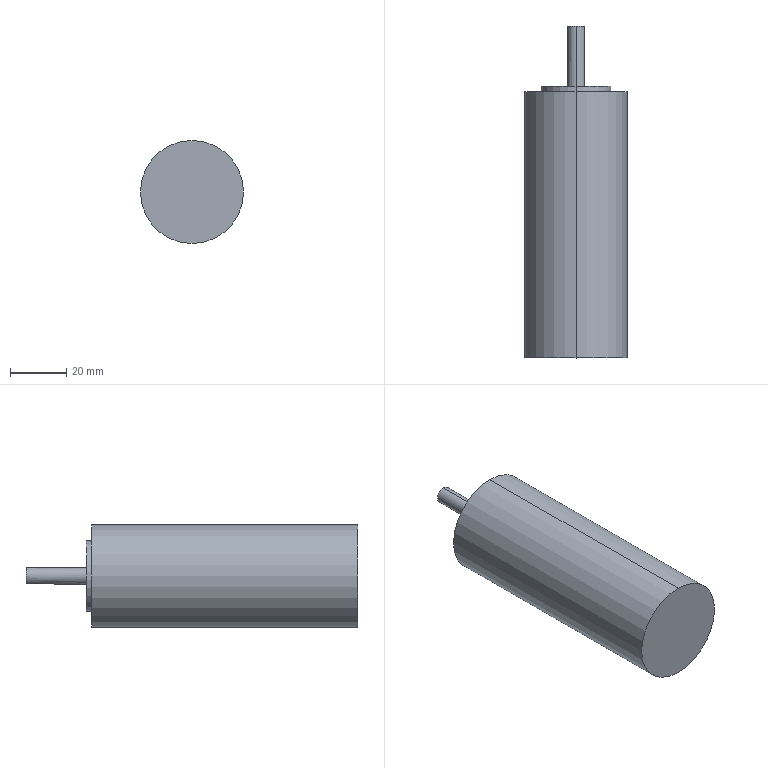Part | 1 solid | 12 faces | box 36.8 x 118.5 x 36.8 mm | volume 102622 mm3 | cylinder 6 | plane 6 | commonest cylinder face diameters 6 x2 25 x2 36.8 x2
STEP:
#1=CARTESIAN_POINT('',(0.,97.,12.5));
#2=VERTEX_POINT('',#1);
#3=CARTESIAN_POINT('',(0.,97.,-12.5));
#4=VERTEX_POINT('',#3);
#5=CARTESIAN_POINT('',(0.,97.,0.));
#6=DIRECTION('',(0.,1.,0.));
#7=DIRECTION('',(0.,0.,1.));
#8=AXIS2_PLACEMENT_3D('',#5,#6,#7);
#9=CIRCLE('',#8,12.5);
#10=EDGE_CURVE('',#2,#4,#9,.T.);
#11=ORIENTED_EDGE('',*,*,#10,.F.);
#12=CARTESIAN_POINT('',(0.,95.,12.5));
#13=VERTEX_POINT('',#12);
#14=CARTESIAN_POINT('',(0.,97.,12.5));
#15=DIRECTION('',(0.,-1.,0.));
#16=VECTOR('',#15,1000.);
#17=LINE('',#14,#16);
#18=EDGE_CURVE('',#2,#13,#17,.T.);
#19=ORIENTED_EDGE('',*,*,#18,.T.);
#20=CARTESIAN_POINT('',(0.,95.,-12.5));
#21=VERTEX_POINT('',#20);
#22=CARTESIAN_POINT('',(0.,95.,0.));
#23=DIRECTION('',(0.,1.,0.));
#24=DIRECTION('',(0.,0.,1.));
#25=AXIS2_PLACEMENT_3D('',#22,#23,#24);
#26=CIRCLE('',#25,12.5);
#27=EDGE_CURVE('',#13,#21,#26,.T.);
#28=ORIENTED_EDGE('',*,*,#27,.T.);
#29=CARTESIAN_POINT('',(0.,97.,-12.5));
#30=DIRECTION('',(0.,-1.,0.));
#31=VECTOR('',#30,1000.);
#32=LINE('',#29,#31);
#33=EDGE_CURVE('',#4,#21,#32,.T.);
#34=ORIENTED_EDGE('',*,*,#33,.F.);
#35=EDGE_LOOP('',(#11,#19,#28,#34));
#36=FACE_OUTER_BOUND('',#35,.T.);
#37=CARTESIAN_POINT('',(0.,97.,0.));
#38=DIRECTION('',(0.,-1.,0.));
#39=DIRECTION('',(0.,0.,-1.));
#40=AXIS2_PLACEMENT_3D('',#37,#38,#39);
#41=CYLINDRICAL_SURFACE('',#40,12.5);
#42=ADVANCED_FACE('',(#36),#41,.T.);
#43=CARTESIAN_POINT('',(0.,95.,18.4));
#44=VERTEX_POINT('',#43);
#45=CARTESIAN_POINT('',(0.,95.,-18.4));
#46=VERTEX_POINT('',#45);
#47=CARTESIAN_POINT('',(0.,95.,0.));
#48=DIRECTION('',(0.,1.,0.));
#49=DIRECTION('',(0.,0.,1.));
#50=AXIS2_PLACEMENT_3D('',#47,#48,#49);
#51=CIRCLE('',#50,18.4);
#52=EDGE_CURVE('',#44,#46,#51,.T.);
#53=ORIENTED_EDGE('',*,*,#52,.F.);
#54=CARTESIAN_POINT('',(0.,0.,18.4));
#55=VERTEX_POINT('',#54);
#56=CARTESIAN_POINT('',(0.,95.,18.4));
#57=DIRECTION('',(0.,-1.,0.));
#58=VECTOR('',#57,1000.);
#59=LINE('',#56,#58);
#60=EDGE_CURVE('',#44,#55,#59,.T.);
#61=ORIENTED_EDGE('',*,*,#60,.T.);
#62=CARTESIAN_POINT('',(0.,0.,-18.4));
#63=VERTEX_POINT('',#62);
#64=CARTESIAN_POINT('',(0.,0.,0.));
#65=DIRECTION('',(0.,1.,0.));
#66=DIRECTION('',(0.,0.,1.));
#67=AXIS2_PLACEMENT_3D('',#64,#65,#66);
#68=CIRCLE('',#67,18.4);
#69=EDGE_CURVE('',#55,#63,#68,.T.);
#70=ORIENTED_EDGE('',*,*,#69,.T.);
#71=CARTESIAN_POINT('',(0.,95.,-18.4));
#72=DIRECTION('',(0.,-1.,0.));
#73=VECTOR('',#72,1000.);
#74=LINE('',#71,#73);
#75=EDGE_CURVE('',#46,#63,#74,.T.);
#76=ORIENTED_EDGE('',*,*,#75,.F.);
#77=EDGE_LOOP('',(#53,#61,#70,#76));
#78=FACE_OUTER_BOUND('',#77,.T.);
#79=CARTESIAN_POINT('',(0.,95.,0.));
#80=DIRECTION('',(0.,-1.,0.));
#81=DIRECTION('',(0.,0.,-1.));
#82=AXIS2_PLACEMENT_3D('',#79,#80,#81);
#83=CYLINDRICAL_SURFACE('',#82,18.4);
#84=ADVANCED_FACE('',(#78),#83,.T.);
#85=CARTESIAN_POINT('',(0.,118.5,3.));
#86=VERTEX_POINT('',#85);
#87=CARTESIAN_POINT('',(1.658,118.5,-2.5));
#88=VERTEX_POINT('',#87);
#89=CARTESIAN_POINT('',(0.,118.5,0.));
#90=DIRECTION('',(0.,1.,0.));
#91=DIRECTION('',(0.,0.,1.));
#92=AXIS2_PLACEMENT_3D('',#89,#90,#91);
#93=CIRCLE('',#92,3.);
#94=EDGE_CURVE('',#86,#88,#93,.T.);
#95=ORIENTED_EDGE('',*,*,#94,.F.);
#96=CARTESIAN_POINT('',(0.,97.,3.));
#97=VERTEX_POINT('',#96);
#98=CARTESIAN_POINT('',(0.,118.5,3.));
#99=DIRECTION('',(0.,-1.,0.));
#100=VECTOR('',#99,1000.);
#101=LINE('',#98,#100);
#102=EDGE_CURVE('',#86,#97,#101,.T.);
#103=ORIENTED_EDGE('',*,*,#102,.T.);
#104=CARTESIAN_POINT('',(0.,97.,-3.));
#105=VERTEX_POINT('',#104);
#106=CARTESIAN_POINT('',(0.,97.,0.));
#107=DIRECTION('',(0.,1.,0.));
#108=DIRECTION('',(0.,0.,1.));
#109=AXIS2_PLACEMENT_3D('',#106,#107,#108);
#110=CIRCLE('',#109,3.);
#111=EDGE_CURVE('',#97,#105,#110,.T.);
#112=ORIENTED_EDGE('',*,*,#111,.T.);
#113=CARTESIAN_POINT('',(0.,108.5,-3.));
#114=VERTEX_POINT('',#113);
#115=CARTESIAN_POINT('',(0.,118.5,-3.));
#116=DIRECTION('',(0.,-1.,0.));
#117=VECTOR('',#116,1000.);
#118=LINE('',#115,#117);
#119=EDGE_CURVE('',#114,#105,#118,.T.);
#120=ORIENTED_EDGE('',*,*,#119,.F.);
#121=CARTESIAN_POINT('',(1.658,108.5,-2.5));
#122=VERTEX_POINT('',#121);
#123=CARTESIAN_POINT('',(0.,108.5,0.));
#124=DIRECTION('',(0.,1.,0.));
#125=DIRECTION('',(0.,0.,1.));
#126=AXIS2_PLACEMENT_3D('',#123,#124,#125);
#127=CIRCLE('',#126,3.);
#128=EDGE_CURVE('',#122,#114,#127,.T.);
#129=ORIENTED_EDGE('',*,*,#128,.F.);
#130=CARTESIAN_POINT('',(1.658,108.5,-2.5));
#131=DIRECTION('',(0.,1.,0.));
#132=VECTOR('',#131,1000.);
#133=LINE('',#130,#132);
#134=EDGE_CURVE('',#122,#88,#133,.T.);
#135=ORIENTED_EDGE('',*,*,#134,.T.);
#136=EDGE_LOOP('',(#95,#103,#112,#120,#129,#135));
#137=FACE_OUTER_BOUND('',#136,.T.);
#138=CARTESIAN_POINT('',(0.,118.5,0.));
#139=DIRECTION('',(0.,-1.,0.));
#140=DIRECTION('',(0.,0.,-1.));
#141=AXIS2_PLACEMENT_3D('',#138,#139,#140);
#142=CYLINDRICAL_SURFACE('',#141,3.);
#143=ADVANCED_FACE('',(#137),#142,.T.);
#144=ORIENTED_EDGE('',*,*,#102,.F.);
#145=CARTESIAN_POINT('',(-1.658,118.5,-2.5));
#146=VERTEX_POINT('',#145);
#147=CARTESIAN_POINT('',(0.,118.5,0.));
#148=DIRECTION('',(0.,1.,0.));
#149=DIRECTION('',(0.,0.,1.));
#150=AXIS2_PLACEMENT_3D('',#147,#148,#149);
#151=CIRCLE('',#150,3.);
#152=EDGE_CURVE('',#146,#86,#151,.T.);
#153=ORIENTED_EDGE('',*,*,#152,.F.);
#154=CARTESIAN_POINT('',(-1.658,108.5,-2.5));
#155=VERTEX_POINT('',#154);
#156=CARTESIAN_POINT('',(-1.658,108.5,-2.5));
#157=DIRECTION('',(0.,1.,0.));
#158=VECTOR('',#157,1000.);
#159=LINE('',#156,#158);
#160=EDGE_CURVE('',#155,#146,#159,.T.);
#161=ORIENTED_EDGE('',*,*,#160,.F.);
#162=CARTESIAN_POINT('',(0.,108.5,0.));
#163=DIRECTION('',(0.,1.,0.));
#164=DIRECTION('',(0.,0.,1.));
#165=AXIS2_PLACEMENT_3D('',#162,#163,#164);
#166=CIRCLE('',#165,3.);
#167=EDGE_CURVE('',#114,#155,#166,.T.);
#168=ORIENTED_EDGE('',*,*,#167,.F.);
#169=ORIENTED_EDGE('',*,*,#119,.T.);
#170=CARTESIAN_POINT('',(0.,97.,0.));
#171=DIRECTION('',(0.,1.,0.));
#172=DIRECTION('',(0.,0.,1.));
#173=AXIS2_PLACEMENT_3D('',#170,#171,#172);
#174=CIRCLE('',#173,3.);
#175=EDGE_CURVE('',#105,#97,#174,.T.);
#176=ORIENTED_EDGE('',*,*,#175,.T.);
#177=EDGE_LOOP('',(#144,#153,#161,#168,#169,#176));
#178=FACE_OUTER_BOUND('',#177,.T.);
#179=CARTESIAN_POINT('',(0.,118.5,0.));
#180=DIRECTION('',(0.,-1.,0.));
#181=DIRECTION('',(0.,0.,-1.));
#182=AXIS2_PLACEMENT_3D('',#179,#180,#181);
#183=CYLINDRICAL_SURFACE('',#182,3.);
#184=ADVANCED_FACE('',(#178),#183,.T.);
#185=ORIENTED_EDGE('',*,*,#152,.T.);
#186=ORIENTED_EDGE('',*,*,#94,.T.);
#187=CARTESIAN_POINT('',(-1.658,118.5,-2.5));
#188=DIRECTION('',(-1.,0.,0.));
#189=VECTOR('',#188,1000.);
#190=LINE('',#187,#189);
#191=EDGE_CURVE('',#88,#146,#190,.T.);
#192=ORIENTED_EDGE('',*,*,#191,.T.);
#193=EDGE_LOOP('',(#185,#186,#192));
#194=FACE_OUTER_BOUND('',#193,.T.);
#195=CARTESIAN_POINT('',(0.,118.5,0.));
#196=DIRECTION('',(0.,1.,0.));
#197=DIRECTION('',(0.,0.,1.));
#198=AXIS2_PLACEMENT_3D('',#195,#196,#197);
#199=PLANE('',#198);
#200=ADVANCED_FACE('',(#194),#199,.T.);
#201=ORIENTED_EDGE('',*,*,#60,.F.);
#202=CARTESIAN_POINT('',(0.,95.,0.));
#203=DIRECTION('',(0.,1.,0.));
#204=DIRECTION('',(0.,0.,1.));
#205=AXIS2_PLACEMENT_3D('',#202,#203,#204);
#206=CIRCLE('',#205,18.4);
#207=EDGE_CURVE('',#46,#44,#206,.T.);
#208=ORIENTED_EDGE('',*,*,#207,.F.);
#209=ORIENTED_EDGE('',*,*,#75,.T.);
#210=CARTESIAN_POINT('',(0.,0.,0.));
#211=DIRECTION('',(0.,1.,0.));
#212=DIRECTION('',(0.,0.,1.));
#213=AXIS2_PLACEMENT_3D('',#210,#211,#212);
#214=CIRCLE('',#213,18.4);
#215=EDGE_CURVE('',#63,#55,#214,.T.);
#216=ORIENTED_EDGE('',*,*,#215,.T.);
#217=EDGE_LOOP('',(#201,#208,#209,#216));
#218=FACE_OUTER_BOUND('',#217,.T.);
#219=CARTESIAN_POINT('',(0.,95.,0.));
#220=DIRECTION('',(0.,-1.,0.));
#221=DIRECTION('',(0.,0.,-1.));
#222=AXIS2_PLACEMENT_3D('',#219,#220,#221);
#223=CYLINDRICAL_SURFACE('',#222,18.4);
#224=ADVANCED_FACE('',(#218),#223,.T.);
#225=CARTESIAN_POINT('',(0.,95.,0.));
#226=DIRECTION('',(0.,1.,0.));
#227=DIRECTION('',(0.,0.,1.));
#228=AXIS2_PLACEMENT_3D('',#225,#226,#227);
#229=CIRCLE('',#228,12.5);
#230=EDGE_CURVE('',#21,#13,#229,.T.);
#231=ORIENTED_EDGE('',*,*,#230,.F.);
#232=ORIENTED_EDGE('',*,*,#27,.F.);
#233=EDGE_LOOP('',(#231,#232));
#234=FACE_BOUND('',#233,.T.);
#235=ORIENTED_EDGE('',*,*,#207,.T.);
#236=ORIENTED_EDGE('',*,*,#52,.T.);
#237=EDGE_LOOP('',(#235,#236));
#238=FACE_OUTER_BOUND('',#237,.T.);
#239=CARTESIAN_POINT('',(0.,95.,0.));
#240=DIRECTION('',(0.,1.,0.));
#241=DIRECTION('',(0.,0.,1.));
#242=AXIS2_PLACEMENT_3D('',#239,#240,#241);
#243=PLANE('',#242);
#244=ADVANCED_FACE('',(#234,#238),#243,.T.);
#245=ORIENTED_EDGE('',*,*,#215,.F.);
#246=ORIENTED_EDGE('',*,*,#69,.F.);
#247=EDGE_LOOP('',(#245,#246));
#248=FACE_OUTER_BOUND('',#247,.T.);
#249=CARTESIAN_POINT('',(0.,0.,0.));
#250=DIRECTION('',(0.,1.,0.));
#251=DIRECTION('',(0.,0.,1.));
#252=AXIS2_PLACEMENT_3D('',#249,#250,#251);
#253=PLANE('',#252);
#254=ADVANCED_FACE('',(#248),#253,.F.);
#255=ORIENTED_EDGE('',*,*,#18,.F.);
#256=CARTESIAN_POINT('',(0.,97.,0.));
#257=DIRECTION('',(0.,1.,0.));
#258=DIRECTION('',(0.,0.,1.));
#259=AXIS2_PLACEMENT_3D('',#256,#257,#258);
#260=CIRCLE('',#259,12.5);
#261=EDGE_CURVE('',#4,#2,#260,.T.);
#262=ORIENTED_EDGE('',*,*,#261,.F.);
#263=ORIENTED_EDGE('',*,*,#33,.T.);
#264=ORIENTED_EDGE('',*,*,#230,.T.);
#265=EDGE_LOOP('',(#255,#262,#263,#264));
#266=FACE_OUTER_BOUND('',#265,.T.);
#267=CARTESIAN_POINT('',(0.,97.,0.));
#268=DIRECTION('',(0.,-1.,0.));
#269=DIRECTION('',(0.,0.,-1.));
#270=AXIS2_PLACEMENT_3D('',#267,#268,#269);
#271=CYLINDRICAL_SURFACE('',#270,12.5);
#272=ADVANCED_FACE('',(#266),#271,.T.);
#273=ORIENTED_EDGE('',*,*,#175,.F.);
#274=ORIENTED_EDGE('',*,*,#111,.F.);
#275=EDGE_LOOP('',(#273,#274));
#276=FACE_BOUND('',#275,.T.);
#277=ORIENTED_EDGE('',*,*,#261,.T.);
#278=ORIENTED_EDGE('',*,*,#10,.T.);
#279=EDGE_LOOP('',(#277,#278));
#280=FACE_OUTER_BOUND('',#279,.T.);
#281=CARTESIAN_POINT('',(0.,97.,0.));
#282=DIRECTION('',(0.,1.,0.));
#283=DIRECTION('',(0.,0.,1.));
#284=AXIS2_PLACEMENT_3D('',#281,#282,#283);
#285=PLANE('',#284);
#286=ADVANCED_FACE('',(#276,#280),#285,.T.);
#287=ORIENTED_EDGE('',*,*,#128,.T.);
#288=ORIENTED_EDGE('',*,*,#167,.T.);
#289=CARTESIAN_POINT('',(-1.658,108.5,-2.5));
#290=DIRECTION('',(-1.,0.,0.));
#291=VECTOR('',#290,1000.);
#292=LINE('',#289,#291);
#293=EDGE_CURVE('',#122,#155,#292,.T.);
#294=ORIENTED_EDGE('',*,*,#293,.F.);
#295=EDGE_LOOP('',(#287,#288,#294));
#296=FACE_OUTER_BOUND('',#295,.T.);
#297=CARTESIAN_POINT('',(0.,108.5,0.));
#298=DIRECTION('',(0.,1.,0.));
#299=DIRECTION('',(0.,0.,1.));
#300=AXIS2_PLACEMENT_3D('',#297,#298,#299);
#301=PLANE('',#300);
#302=ADVANCED_FACE('',(#296),#301,.T.);
#303=ORIENTED_EDGE('',*,*,#191,.F.);
#304=ORIENTED_EDGE('',*,*,#134,.F.);
#305=ORIENTED_EDGE('',*,*,#293,.T.);
#306=ORIENTED_EDGE('',*,*,#160,.T.);
#307=EDGE_LOOP('',(#303,#304,#305,#306));
#308=FACE_OUTER_BOUND('',#307,.T.);
#309=CARTESIAN_POINT('',(-1.658,108.5,-2.5));
#310=DIRECTION('',(0.,0.,-1.));
#311=DIRECTION('',(-1.,0.,0.));
#312=AXIS2_PLACEMENT_3D('',#309,#310,#311);
#313=PLANE('',#312);
#314=ADVANCED_FACE('',(#308),#313,.T.);
#315=CLOSED_SHELL('',(#42,#84,#143,#184,#200,#224,#244,#254,#272,#286,#302,#314));
#316=MANIFOLD_SOLID_BREP('',#315);
#317=CARTESIAN_POINT('',(0.,0.,0.));
#318=DIRECTION('',(0.,0.,1.));
#319=DIRECTION('',(1.,0.,0.));
#320=AXIS2_PLACEMENT_3D('',#317,#318,#319);
#321=(LENGTH_UNIT()NAMED_UNIT(*)SI_UNIT(.MILLI.,.METRE.));
#322=UNCERTAINTY_MEASURE_WITH_UNIT(LENGTH_MEASURE(0.00001),#321,'','');
#323=(NAMED_UNIT(*)PLANE_ANGLE_UNIT()SI_UNIT($,.RADIAN.));
#324=(NAMED_UNIT(*)SI_UNIT($,.STERADIAN.)SOLID_ANGLE_UNIT());
#325=(GEOMETRIC_REPRESENTATION_CONTEXT(3)GLOBAL_UNCERTAINTY_ASSIGNED_CONTEXT((#322))GLOBAL_UNIT_ASSIGNED_CONTEXT((#321,#323,#324))REPRESENTATION_CONTEXT('',''));
#326=ADVANCED_BREP_SHAPE_REPRESENTATION('',(#316,#320),#325);